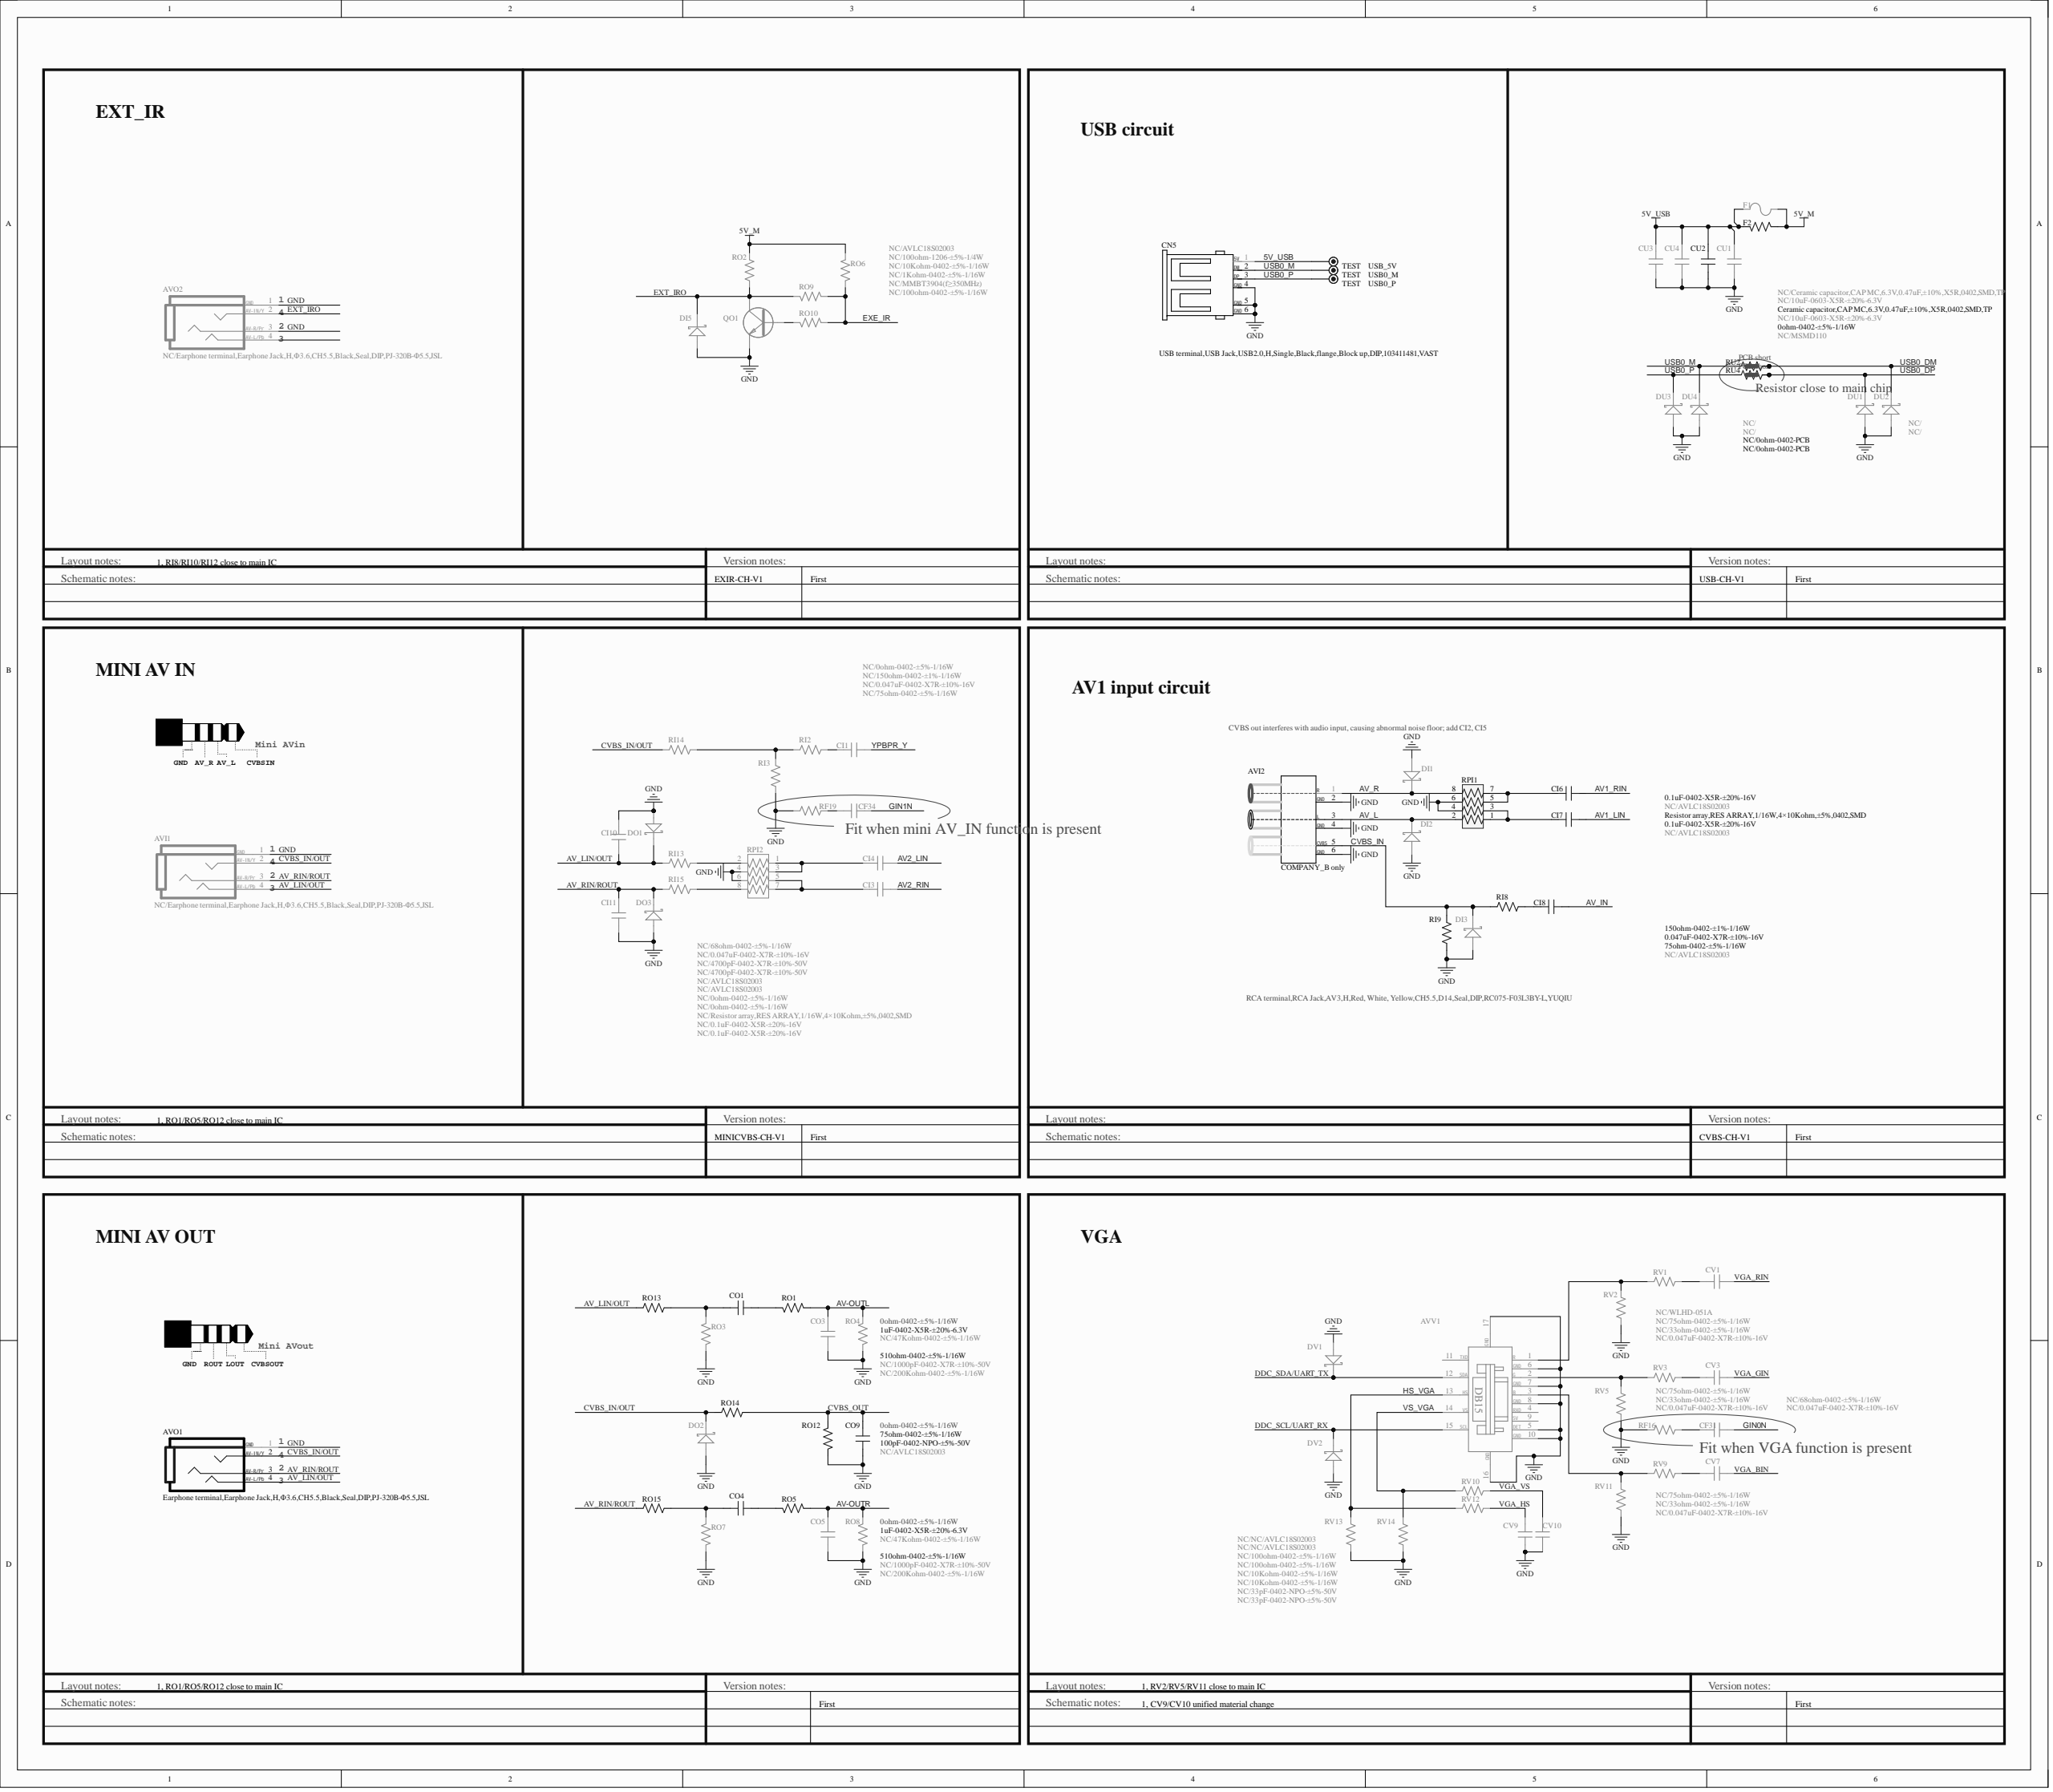Circuit board | Altium Designer | 574 parts | 274 nets | one sheet of the schematic
Parts on this sheet (reference | value | footprint):
AVI1 | NC/Earphone terminal,Earphone Jack,H,F3.6,CH5.5,Black,Seal,DIP,PJ-320B-F5.5,JSL | PHONE-HD-43
AVI2 | RCA terminal,RCA Jack,AV3,H,Red, White, Yellow,CH5.5,D14,Seal,DIP,RC075-F03L3BY-L,YUQIU | AV3-H14-15
AVO1 | Earphone terminal,Earphone Jack,H,F3.6,CH5.5,Black,Seal,DIP,PJ-320B-F5.5,JSL | PHONE-HD-43
AVO2 | NC/Earphone terminal,Earphone Jack,H,F3.6,CH5.5,Black,Seal,DIP,PJ-320B-F5.5,JSL | PHONE-HD-43
AVV1 | NC/WLHD-051A | DB15-HF-1
CF31 | NC/0.047uF-0402-X7R-±10%-16V | C0402
CF34 | NC/0.047uF-0402-X7R-±10%-16V | C0402
CI1 | NC/0.047uF-0402-X7R-±10%-16V | C0402
CI3 | NC/0.1uF-0402-X5R-±20%-16V | C0402
CI4 | NC/0.1uF-0402-X5R-±20%-16V | C0402
CI6 | 0.1uF-0402-X5R-±20%-16V | C0402
CI7 | 0.1uF-0402-X5R-±20%-16V | C0402
CI8 | 0.047uF-0402-X7R-±10%-16V | C0402
CI10 | NC/4700pF-0402-X7R-±10%-50V | C0402
CI11 | NC/4700pF-0402-X7R-±10%-50V | C0402
CN5 | USB terminal,USB Jack,USB2.0,H,Single,Black,flange,Block up,DIP,103411481,VAST | USB-HD-30
CO1 | 1uF-0402-X5R-±20%-6.3V | C0402
CO3 | NC/1000pF-0402-X7R-±10%-50V | C0402
CO4 | 1uF-0402-X5R-±20%-6.3V | C0402
CO5 | NC/1000pF-0402-X7R-±10%-50V | C0402
CO9 | 100pF-0402-NPO-±5%-50V | C0402
CU1 | NC/10uF-0603-X5R-±20%-6.3V | C0603
CU2 | Ceramic capacitor,CAP MC,6.3V,0.47uF,±10%,X5R,0402,SMD,TP | C0402
CU3 | NC/Ceramic capacitor,CAP MC,6.3V,0.47uF,±10%,X5R,0402,SMD,TP | C0402
CU4 | NC/10uF-0603-X5R-±20%-6.3V | C0603
CV1 | NC/0.047uF-0402-X7R-±10%-16V | C0402
CV3 | NC/0.047uF-0402-X7R-±10%-16V | C0402
CV7 | NC/0.047uF-0402-X7R-±10%-16V | C0402
CV9 | NC/33pF-0402-NPO-±5%-50V | C0402
CV10 | NC/33pF-0402-NPO-±5%-50V | C0402
DI1 | NC/AVLC18S02003 | DIODE-S0402
DI2 | NC/AVLC18S02003 | DIODE-S0402
DI3 | NC/AVLC18S02003 | DIODE-S0402
DI5 | NC/AVLC18S02003 | DIODE-S0402
DO1 | NC/AVLC18S02003 | DIODE-S0402
DO2 | NC/AVLC18S02003 | DIODE-S0402
DO3 | NC/AVLC18S02003 | DIODE-S0402
DU1 | NC/ | DIODE-S0402
DU2 | NC/ | DIODE-S0402
DU3 | NC/ | DIODE-S0402
DU4 | NC/ | DIODE-S0402
DV1 | NC/NC/AVLC18S02003 | DIODE-S0402
DV2 | NC/NC/AVLC18S02003 | DIODE-S0402
F1 | NC/MSMD110 | FUSE3.5A-S
F2 | 0ohm-0402-±5%-1/16W | R0402
QO1 | NC/MMBT3904(f=350MHz) | SOT-23
RF16 | NC/68ohm-0402-±5%-1/16W | R0402
RF19 | NC/68ohm-0402-±5%-1/16W | R0402
RI2 | NC/150ohm-0402-±1%-1/16W | R0402
RI3 | NC/75ohm-0402-±5%-1/16W | R0402
RI8 | 150ohm-0402-±1%-1/16W | R0402
RI9 | 75ohm-0402-±5%-1/16W | R0402
RI13 | NC/0ohm-0402-±5%-1/16W | R0402
RI14 | NC/0ohm-0402-±5%-1/16W | R0402
RI15 | NC/0ohm-0402-±5%-1/16W | R0402
RO1 | 510ohm-0402-±5%-1/16W | R0402
RO2 | NC/100ohm-1206-±5%-1/4W | R1206
RO3 | NC/47Kohm-0402-±5%-1/16W | R0402
RO4 | NC/200Kohm-0402-±5%-1/16W | R0402
RO5 | 510ohm-0402-±5%-1/16W | R0402
RO6 | NC/10Kohm-0402-±5%-1/16W | R0402
RO7 | NC/47Kohm-0402-±5%-1/16W | R0402
RO8 | NC/200Kohm-0402-±5%-1/16W | R0402
RO9 | NC/100ohm-0402-±5%-1/16W | R0402
RO10 | NC/1Kohm-0402-±5%-1/16W | R0402
RO12 | 75ohm-0402-±5%-1/16W | R0402
RO13 | 0ohm-0402-±5%-1/16W | R0402
RO14 | 0ohm-0402-±5%-1/16W | R0402
RO15 | 0ohm-0402-±5%-1/16W | R0402
RPI1 | Resistor array,RES ARRAY,1/16W,4×10Kohm,±5%,0402,SMD | RA0402
RPI2 | NC/Resistor array,RES ARRAY,1/16W,4×10Kohm,±5%,0402,SMD | RA0402
RU2 | NC/0ohm-0402-PCB | R0402SC
RU4 | NC/0ohm-0402-PCB | R0402SC
RV1 | NC/33ohm-0402-±5%-1/16W | R0402
RV2 | NC/75ohm-0402-±5%-1/16W | R0402
RV3 | NC/33ohm-0402-±5%-1/16W | R0402
RV5 | NC/75ohm-0402-±5%-1/16W | R0402
RV9 | NC/33ohm-0402-±5%-1/16W | R0402
RV10 | NC/100ohm-0402-±5%-1/16W | R0402
RV11 | NC/75ohm-0402-±5%-1/16W | R0402
RV12 | NC/100ohm-0402-±5%-1/16W | R0402
RV13 | NC/10Kohm-0402-±5%-1/16W | R0402
RV14 | NC/10Kohm-0402-±5%-1/16W | R0402
USB0_M | TEST | TP
USB0_P | TEST | TP
USB_5V | TEST | TP
Nets of these parts (net: part-pin ...):
YPBPR_Y: CI1-1
VS_VGA: AVV1-14 RV10-1 RV14-1
VGA_VS: CV10-2 RV10-2
VGA_RIN: CV1-1
VGA_HS: CV9-2 RV12-2
VGA_GIN: CV3-1
VGA_BIN: CV7-1
USB0_P: CN5-3 DU3-K RU4-1 USB0_P-1
USB0_M: CN5-2 DU4-K RU2-1 USB0_M-1
USB0_DP: DU1-K RU4-2 RU4-3
USB0_DM: DU2-K RU2-2 RU2-3
NetRI15_2: RI15-2 RPI2-8
NetRI13_2: RI13-2 RPI2-2
NetRI2_1: RI2-1 RI3-2 RI14-2
NetQO1_B: QO1-B RO10-1
NetCV7_2: CV7-2 RV9-1
NetCV3_2: CV3-2 RV3-1
NetCV1_2: CV1-2 RV1-1
NetCO4_2: CO4-2 RO5-2
NetCO4_1: CO4-1 RO7-2 RO15-2
NetCO1_2: CO1-2 RO1-2
NetCO1_1: CO1-1 RO3-2 RO13-2
NetCI8_2: CI8-2 RI8-2
NetCI7_2: CI7-2 RPI1-1 RPI1-3
NetCI6_2: CI6-2 RPI1-5 RPI1-7
NetCI4_2: CI4-2 RPI2-1 RPI2-3
NetCI3_2: CI3-2 RPI2-5 RPI2-7
NetCI1_2: CI1-2 RI2-2
NetCF34_1: CF34-1 RF19-2
NetCF31_2: CF31-2 RF16-1
NetAVV1_3: AVV1-3 RV9-2 RV11-2
NetAVV1_2: AVV1-2 RV3-2 RV5-2
NetAVV1_1: AVV1-1 RV1-2 RV2-2
HS_VGA: AVV1-13 RV12-1 RV13-1
GND: AVI1-1 AVI2-2 AVI2-4 AVI2-6 AVO1-1 AVO2-1 AVO2-3 AVV1-5 AVV1-6 AVV1-7 AVV1-8 AVV1-10 AVV1-16 AVV1-17 CI10-2 CI11-2 CN5-4 CN5-5 CN5-6 CO3-1 CO5-1 CO9-1 CU1-1 CU2-2 CU3-2 CU4-1 CV9-1 CV10-1 DI1-A DI2-A DI3-A DI5-A DO1-A DO2-A DO3-A DU1-A DU2-A DU3-A DU4-A DV1-A DV2-A QO1-E RF16-2 RF19-1 RI3-1 RI9-1 RO3-1 RO4-1 RO7-1 RO8-1 RO12-2 RPI1-4 RPI1-6 RPI2-4 RPI2-6 RV2-1 RV5-1 RV11-1 RV13-2 RV14-2
GIN1N: CF34-2
GIN0N: CF31-1
EXT_IRO: AVO2-2 DI5-K QO1-C RO2-1 RO9-1
EXE_IR: RO6-2 RO9-2 RO10-2
DDC_SDA/UART_TX: AVV1-12 DV1-K
DDC_SCL/UART_RX: AVV1-15 DV2-K
CVBS_OUT: CO9-2 RO12-1 RO14-2
CVBS_IN/OUT: AVI1-2 AVO1-2 DO2-K RI14-1 RO14-1
CVBS_IN: AVI2-5 DI3-K RI8-1 RI9-2
AV_RIN/ROUT: AVI1-3 AVO1-3 CI11-1 DO3-K RI15-1 RO15-1
AV_R: AVI2-1 DI1-K RPI1-8
AV_LIN/OUT: AVI1-4 AVO1-4 CI10-1 DO1-K RI13-1 RO13-1
AV_L: AVI2-3 DI2-K RPI1-2
AV_IN: CI8-1
AV-OUTR: CO5-2 RO5-1 RO8-2
AV-OUTL: CO3-2 RO1-1 RO4-2
AV2_RIN: CI3-1
AV2_LIN: CI4-1
AV1_RIN: CI6-1
AV1_LIN: CI7-1
5V_USB: CN5-1 CU1-2 CU2-1 CU3-1 CU4-2 F1-1 F2-2 USB_5V-1
5V_M: F1-2 F2-1 RO2-2 RO6-1